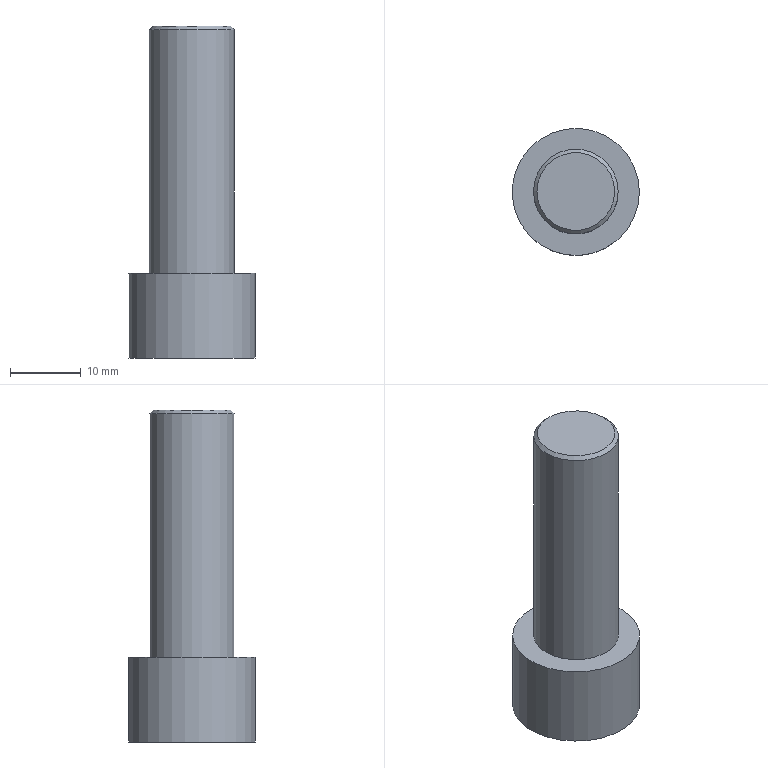Part | STEP file | 1_id58_xmt_txt | 1 solid | 19 faces | box 18 x 18 x 47 mm | volume 6453 mm3 | plane 15 | cylinder 2 | cone 2 | commonest cylinder face diameters 12 x1 18 x1
STEP:
#1=CARTESIAN_POINT('',(86.,-23.,-79.));
#2=VERTEX_POINT('',#1);
#3=CARTESIAN_POINT('',(77.,-23.,-79.));
#4=DIRECTION('',(0.,0.,-1.));
#5=DIRECTION('',(1.,0.,0.));
#6=AXIS2_PLACEMENT_3D('',#3,#4,#5);
#7=CIRCLE('',#6,9.);
#8=EDGE_CURVE('',#2,#2,#7,.T.);
#9=ORIENTED_EDGE('',*,*,#8,.F.);
#10=EDGE_LOOP('',(#9));
#11=FACE_BOUND('',#10,.T.);
#12=CARTESIAN_POINT('',(86.,-23.,-67.));
#13=VERTEX_POINT('',#12);
#14=CARTESIAN_POINT('',(77.,-23.,-67.));
#15=DIRECTION('',(0.,0.,1.));
#16=DIRECTION('',(1.,0.,0.));
#17=AXIS2_PLACEMENT_3D('',#14,#15,#16);
#18=CIRCLE('',#17,9.);
#19=EDGE_CURVE('',#13,#13,#18,.T.);
#20=ORIENTED_EDGE('',*,*,#19,.F.);
#21=EDGE_LOOP('',(#20));
#22=FACE_BOUND('',#21,.T.);
#23=CARTESIAN_POINT('',(77.,-23.,-73.));
#24=DIRECTION('',(0.,0.,1.));
#25=DIRECTION('',(-1.,0.,0.));
#26=AXIS2_PLACEMENT_3D('',#23,#24,#25);
#27=CYLINDRICAL_SURFACE('',#26,9.);
#28=ADVANCED_FACE('',(#11,#22),#27,.T.);
#29=CARTESIAN_POINT('',(77.,-17.226,-73.));
#30=VERTEX_POINT('',#29);
#31=CARTESIAN_POINT('',(82.,-20.113,-73.));
#32=VERTEX_POINT('',#31);
#33=CARTESIAN_POINT('',(77.,-23.,-73.));
#34=DIRECTION('',(0.,0.,-1.));
#35=DIRECTION('',(1.,0.,0.));
#36=AXIS2_PLACEMENT_3D('',#33,#34,#35);
#37=CIRCLE('',#36,5.774);
#38=EDGE_CURVE('',#30,#32,#37,.T.);
#39=ORIENTED_EDGE('',*,*,#38,.T.);
#40=CARTESIAN_POINT('',(82.,-25.887,-73.));
#41=VERTEX_POINT('',#40);
#42=CARTESIAN_POINT('',(77.,-23.,-73.));
#43=DIRECTION('',(0.,0.,-1.));
#44=DIRECTION('',(1.,0.,0.));
#45=AXIS2_PLACEMENT_3D('',#42,#43,#44);
#46=CIRCLE('',#45,5.774);
#47=EDGE_CURVE('',#32,#41,#46,.T.);
#48=ORIENTED_EDGE('',*,*,#47,.T.);
#49=CARTESIAN_POINT('',(77.,-28.774,-73.));
#50=VERTEX_POINT('',#49);
#51=CARTESIAN_POINT('',(77.,-23.,-73.));
#52=DIRECTION('',(0.,0.,-1.));
#53=DIRECTION('',(1.,0.,0.));
#54=AXIS2_PLACEMENT_3D('',#51,#52,#53);
#55=CIRCLE('',#54,5.774);
#56=EDGE_CURVE('',#41,#50,#55,.T.);
#57=ORIENTED_EDGE('',*,*,#56,.T.);
#58=CARTESIAN_POINT('',(72.,-25.887,-73.));
#59=VERTEX_POINT('',#58);
#60=CARTESIAN_POINT('',(77.,-23.,-73.));
#61=DIRECTION('',(0.,0.,-1.));
#62=DIRECTION('',(1.,0.,0.));
#63=AXIS2_PLACEMENT_3D('',#60,#61,#62);
#64=CIRCLE('',#63,5.774);
#65=EDGE_CURVE('',#50,#59,#64,.T.);
#66=ORIENTED_EDGE('',*,*,#65,.T.);
#67=CARTESIAN_POINT('',(72.,-20.113,-73.));
#68=VERTEX_POINT('',#67);
#69=CARTESIAN_POINT('',(77.,-23.,-73.));
#70=DIRECTION('',(0.,0.,-1.));
#71=DIRECTION('',(1.,0.,0.));
#72=AXIS2_PLACEMENT_3D('',#69,#70,#71);
#73=CIRCLE('',#72,5.774);
#74=EDGE_CURVE('',#59,#68,#73,.T.);
#75=ORIENTED_EDGE('',*,*,#74,.T.);
#76=CARTESIAN_POINT('',(77.,-23.,-73.));
#77=DIRECTION('',(0.,0.,-1.));
#78=DIRECTION('',(1.,0.,0.));
#79=AXIS2_PLACEMENT_3D('',#76,#77,#78);
#80=CIRCLE('',#79,5.774);
#81=EDGE_CURVE('',#68,#30,#80,.T.);
#82=ORIENTED_EDGE('',*,*,#81,.T.);
#83=EDGE_LOOP('',(#39,#48,#57,#66,#75,#82));
#84=FACE_BOUND('',#83,.T.);
#85=CARTESIAN_POINT('',(77.,-23.,-72.));
#86=VERTEX_POINT('',#85);
#87=VERTEX_LOOP('',#86);
#88=FACE_BOUND('',#87,.T.);
#89=CARTESIAN_POINT('',(77.,-23.,-72.5));
#90=DIRECTION('',(0.,0.,-1.));
#91=DIRECTION('',(-1.,0.,0.));
#92=AXIS2_PLACEMENT_3D('',#89,#90,#91);
#93=CONICAL_SURFACE('',#92,2.887,80.174);
#94=ADVANCED_FACE('',(#84,#88),#93,.F.);
#95=CARTESIAN_POINT('',(83.,-23.,-67.));
#96=VERTEX_POINT('',#95);
#97=CARTESIAN_POINT('',(77.,-23.,-67.));
#98=DIRECTION('',(0.,0.,-1.));
#99=DIRECTION('',(1.,0.,0.));
#100=AXIS2_PLACEMENT_3D('',#97,#98,#99);
#101=CIRCLE('',#100,6.);
#102=EDGE_CURVE('',#96,#96,#101,.T.);
#103=ORIENTED_EDGE('',*,*,#102,.F.);
#104=EDGE_LOOP('',(#103));
#105=FACE_BOUND('',#104,.T.);
#106=CARTESIAN_POINT('',(71.,-23.,-32.5));
#107=VERTEX_POINT('',#106);
#108=CARTESIAN_POINT('',(77.,-23.,-32.5));
#109=DIRECTION('',(0.,0.,1.));
#110=DIRECTION('',(-1.,0.,0.));
#111=AXIS2_PLACEMENT_3D('',#108,#109,#110);
#112=CIRCLE('',#111,6.);
#113=EDGE_CURVE('',#107,#107,#112,.T.);
#114=ORIENTED_EDGE('',*,*,#113,.F.);
#115=EDGE_LOOP('',(#114));
#116=FACE_BOUND('',#115,.T.);
#117=CARTESIAN_POINT('',(77.,-23.,-49.5));
#118=DIRECTION('',(0.,0.,1.));
#119=DIRECTION('',(-1.,0.,0.));
#120=AXIS2_PLACEMENT_3D('',#117,#118,#119);
#121=CYLINDRICAL_SURFACE('',#120,6.);
#122=ADVANCED_FACE('',(#105,#116),#121,.T.);
#123=ORIENTED_EDGE('',*,*,#113,.T.);
#124=EDGE_LOOP('',(#123));
#125=FACE_BOUND('',#124,.T.);
#126=CARTESIAN_POINT('',(71.5,-23.,-32.));
#127=VERTEX_POINT('',#126);
#128=CARTESIAN_POINT('',(77.,-23.,-32.));
#129=DIRECTION('',(0.,0.,-1.));
#130=DIRECTION('',(-1.,0.,0.));
#131=AXIS2_PLACEMENT_3D('',#128,#129,#130);
#132=CIRCLE('',#131,5.5);
#133=EDGE_CURVE('',#127,#127,#132,.T.);
#134=ORIENTED_EDGE('',*,*,#133,.T.);
#135=EDGE_LOOP('',(#134));
#136=FACE_BOUND('',#135,.T.);
#137=CARTESIAN_POINT('',(77.,-23.,-32.));
#138=DIRECTION('',(0.,0.,-1.));
#139=DIRECTION('',(1.,0.,0.));
#140=AXIS2_PLACEMENT_3D('',#137,#138,#139);
#141=CONICAL_SURFACE('',#140,5.5,45.);
#142=ADVANCED_FACE('',(#125,#136),#141,.T.);
#143=ORIENTED_EDGE('',*,*,#133,.F.);
#144=EDGE_LOOP('',(#143));
#145=FACE_OUTER_BOUND('',#144,.T.);
#146=CARTESIAN_POINT('',(77.,-23.,-32.));
#147=DIRECTION('',(0.,0.,1.));
#148=DIRECTION('',(-1.,0.,0.));
#149=AXIS2_PLACEMENT_3D('',#146,#147,#148);
#150=PLANE('',#149);
#151=ADVANCED_FACE('',(#145),#150,.T.);
#152=CARTESIAN_POINT('',(79.5,-27.33,-73.));
#153=DIRECTION('',(0.866,0.5,0.));
#154=VECTOR('',#153,1.);
#155=LINE('',#152,#154);
#156=EDGE_CURVE('',#50,#41,#155,.T.);
#157=ORIENTED_EDGE('',*,*,#156,.F.);
#158=ORIENTED_EDGE('',*,*,#56,.F.);
#159=EDGE_LOOP('',(#157,#158));
#160=FACE_OUTER_BOUND('',#159,.T.);
#161=CARTESIAN_POINT('',(77.,-23.,-73.));
#162=DIRECTION('',(0.,0.,-1.));
#163=DIRECTION('',(1.,0.,0.));
#164=AXIS2_PLACEMENT_3D('',#161,#162,#163);
#165=PLANE('',#164);
#166=ADVANCED_FACE('',(#160),#165,.F.);
#167=CARTESIAN_POINT('',(82.,-23.,-73.));
#168=DIRECTION('',(0.,1.,0.));
#169=VECTOR('',#168,1.);
#170=LINE('',#167,#169);
#171=EDGE_CURVE('',#41,#32,#170,.T.);
#172=ORIENTED_EDGE('',*,*,#171,.F.);
#173=ORIENTED_EDGE('',*,*,#47,.F.);
#174=EDGE_LOOP('',(#172,#173));
#175=FACE_OUTER_BOUND('',#174,.T.);
#176=CARTESIAN_POINT('',(77.,-23.,-73.));
#177=DIRECTION('',(0.,0.,-1.));
#178=DIRECTION('',(1.,0.,0.));
#179=AXIS2_PLACEMENT_3D('',#176,#177,#178);
#180=PLANE('',#179);
#181=ADVANCED_FACE('',(#175),#180,.F.);
#182=CARTESIAN_POINT('',(79.5,-18.67,-73.));
#183=DIRECTION('',(-0.866,0.5,0.));
#184=VECTOR('',#183,1.);
#185=LINE('',#182,#184);
#186=EDGE_CURVE('',#32,#30,#185,.T.);
#187=ORIENTED_EDGE('',*,*,#186,.F.);
#188=ORIENTED_EDGE('',*,*,#38,.F.);
#189=EDGE_LOOP('',(#187,#188));
#190=FACE_OUTER_BOUND('',#189,.T.);
#191=CARTESIAN_POINT('',(77.,-23.,-73.));
#192=DIRECTION('',(0.,0.,-1.));
#193=DIRECTION('',(1.,0.,0.));
#194=AXIS2_PLACEMENT_3D('',#191,#192,#193);
#195=PLANE('',#194);
#196=ADVANCED_FACE('',(#190),#195,.F.);
#197=CARTESIAN_POINT('',(74.5,-18.67,-73.));
#198=DIRECTION('',(-0.866,-0.5,0.));
#199=VECTOR('',#198,1.);
#200=LINE('',#197,#199);
#201=EDGE_CURVE('',#30,#68,#200,.T.);
#202=ORIENTED_EDGE('',*,*,#201,.F.);
#203=ORIENTED_EDGE('',*,*,#81,.F.);
#204=EDGE_LOOP('',(#202,#203));
#205=FACE_OUTER_BOUND('',#204,.T.);
#206=CARTESIAN_POINT('',(77.,-23.,-73.));
#207=DIRECTION('',(0.,0.,-1.));
#208=DIRECTION('',(1.,0.,0.));
#209=AXIS2_PLACEMENT_3D('',#206,#207,#208);
#210=PLANE('',#209);
#211=ADVANCED_FACE('',(#205),#210,.F.);
#212=CARTESIAN_POINT('',(72.,-23.,-73.));
#213=DIRECTION('',(0.,-1.,0.));
#214=VECTOR('',#213,1.);
#215=LINE('',#212,#214);
#216=EDGE_CURVE('',#68,#59,#215,.T.);
#217=ORIENTED_EDGE('',*,*,#216,.F.);
#218=ORIENTED_EDGE('',*,*,#74,.F.);
#219=EDGE_LOOP('',(#217,#218));
#220=FACE_OUTER_BOUND('',#219,.T.);
#221=CARTESIAN_POINT('',(77.,-23.,-73.));
#222=DIRECTION('',(0.,0.,-1.));
#223=DIRECTION('',(1.,0.,0.));
#224=AXIS2_PLACEMENT_3D('',#221,#222,#223);
#225=PLANE('',#224);
#226=ADVANCED_FACE('',(#220),#225,.F.);
#227=CARTESIAN_POINT('',(74.5,-27.33,-73.));
#228=DIRECTION('',(0.866,-0.5,0.));
#229=VECTOR('',#228,1.);
#230=LINE('',#227,#229);
#231=EDGE_CURVE('',#59,#50,#230,.T.);
#232=ORIENTED_EDGE('',*,*,#231,.F.);
#233=ORIENTED_EDGE('',*,*,#65,.F.);
#234=EDGE_LOOP('',(#232,#233));
#235=FACE_OUTER_BOUND('',#234,.T.);
#236=CARTESIAN_POINT('',(77.,-23.,-73.));
#237=DIRECTION('',(0.,0.,-1.));
#238=DIRECTION('',(1.,0.,0.));
#239=AXIS2_PLACEMENT_3D('',#236,#237,#238);
#240=PLANE('',#239);
#241=ADVANCED_FACE('',(#235),#240,.F.);
#242=CARTESIAN_POINT('',(77.,-28.774,-79.));
#243=VERTEX_POINT('',#242);
#244=CARTESIAN_POINT('',(77.,-28.774,-76.));
#245=DIRECTION('',(0.,0.,-1.));
#246=VECTOR('',#245,1.);
#247=LINE('',#244,#246);
#248=EDGE_CURVE('',#50,#243,#247,.T.);
#249=ORIENTED_EDGE('',*,*,#248,.F.);
#250=ORIENTED_EDGE('',*,*,#156,.T.);
#251=CARTESIAN_POINT('',(82.,-25.887,-79.));
#252=VERTEX_POINT('',#251);
#253=CARTESIAN_POINT('',(82.,-25.887,-76.));
#254=DIRECTION('',(0.,0.,-1.));
#255=VECTOR('',#254,1.);
#256=LINE('',#253,#255);
#257=EDGE_CURVE('',#41,#252,#256,.T.);
#258=ORIENTED_EDGE('',*,*,#257,.T.);
#259=CARTESIAN_POINT('',(79.5,-27.33,-79.));
#260=DIRECTION('',(0.866,0.5,0.));
#261=VECTOR('',#260,1.);
#262=LINE('',#259,#261);
#263=EDGE_CURVE('',#243,#252,#262,.T.);
#264=ORIENTED_EDGE('',*,*,#263,.F.);
#265=EDGE_LOOP('',(#249,#250,#258,#264));
#266=FACE_OUTER_BOUND('',#265,.T.);
#267=CARTESIAN_POINT('',(79.5,-27.33,-76.));
#268=DIRECTION('',(-0.5,0.866,0.));
#269=DIRECTION('',(0.,0.,-1.));
#270=AXIS2_PLACEMENT_3D('',#267,#268,#269);
#271=PLANE('',#270);
#272=ADVANCED_FACE('',(#266),#271,.T.);
#273=CARTESIAN_POINT('',(72.,-25.887,-79.));
#274=VERTEX_POINT('',#273);
#275=CARTESIAN_POINT('',(72.,-25.887,-76.));
#276=DIRECTION('',(0.,0.,-1.));
#277=VECTOR('',#276,1.);
#278=LINE('',#275,#277);
#279=EDGE_CURVE('',#59,#274,#278,.T.);
#280=ORIENTED_EDGE('',*,*,#279,.F.);
#281=ORIENTED_EDGE('',*,*,#231,.T.);
#282=ORIENTED_EDGE('',*,*,#248,.T.);
#283=CARTESIAN_POINT('',(74.5,-27.33,-79.));
#284=DIRECTION('',(0.866,-0.5,0.));
#285=VECTOR('',#284,1.);
#286=LINE('',#283,#285);
#287=EDGE_CURVE('',#274,#243,#286,.T.);
#288=ORIENTED_EDGE('',*,*,#287,.F.);
#289=EDGE_LOOP('',(#280,#281,#282,#288));
#290=FACE_OUTER_BOUND('',#289,.T.);
#291=CARTESIAN_POINT('',(74.5,-27.33,-76.));
#292=DIRECTION('',(0.5,0.866,0.));
#293=DIRECTION('',(0.,0.,1.));
#294=AXIS2_PLACEMENT_3D('',#291,#292,#293);
#295=PLANE('',#294);
#296=ADVANCED_FACE('',(#290),#295,.T.);
#297=CARTESIAN_POINT('',(72.,-20.113,-79.));
#298=VERTEX_POINT('',#297);
#299=CARTESIAN_POINT('',(72.,-20.113,-76.));
#300=DIRECTION('',(0.,0.,-1.));
#301=VECTOR('',#300,1.);
#302=LINE('',#299,#301);
#303=EDGE_CURVE('',#68,#298,#302,.T.);
#304=ORIENTED_EDGE('',*,*,#303,.F.);
#305=ORIENTED_EDGE('',*,*,#216,.T.);
#306=ORIENTED_EDGE('',*,*,#279,.T.);
#307=CARTESIAN_POINT('',(72.,-23.,-79.));
#308=DIRECTION('',(0.,-1.,0.));
#309=VECTOR('',#308,1.);
#310=LINE('',#307,#309);
#311=EDGE_CURVE('',#298,#274,#310,.T.);
#312=ORIENTED_EDGE('',*,*,#311,.F.);
#313=EDGE_LOOP('',(#304,#305,#306,#312));
#314=FACE_OUTER_BOUND('',#313,.T.);
#315=CARTESIAN_POINT('',(72.,-23.,-76.));
#316=DIRECTION('',(1.,0.,0.));
#317=DIRECTION('',(0.,0.,1.));
#318=AXIS2_PLACEMENT_3D('',#315,#316,#317);
#319=PLANE('',#318);
#320=ADVANCED_FACE('',(#314),#319,.T.);
#321=CARTESIAN_POINT('',(77.,-17.226,-79.));
#322=VERTEX_POINT('',#321);
#323=CARTESIAN_POINT('',(77.,-17.226,-76.));
#324=DIRECTION('',(0.,0.,-1.));
#325=VECTOR('',#324,1.);
#326=LINE('',#323,#325);
#327=EDGE_CURVE('',#30,#322,#326,.T.);
#328=ORIENTED_EDGE('',*,*,#327,.F.);
#329=ORIENTED_EDGE('',*,*,#201,.T.);
#330=ORIENTED_EDGE('',*,*,#303,.T.);
#331=CARTESIAN_POINT('',(74.5,-18.67,-79.));
#332=DIRECTION('',(-0.866,-0.5,0.));
#333=VECTOR('',#332,1.);
#334=LINE('',#331,#333);
#335=EDGE_CURVE('',#322,#298,#334,.T.);
#336=ORIENTED_EDGE('',*,*,#335,.F.);
#337=EDGE_LOOP('',(#328,#329,#330,#336));
#338=FACE_OUTER_BOUND('',#337,.T.);
#339=CARTESIAN_POINT('',(74.5,-18.67,-76.));
#340=DIRECTION('',(0.5,-0.866,0.));
#341=DIRECTION('',(0.,0.,1.));
#342=AXIS2_PLACEMENT_3D('',#339,#340,#341);
#343=PLANE('',#342);
#344=ADVANCED_FACE('',(#338),#343,.T.);
#345=CARTESIAN_POINT('',(82.,-20.113,-79.));
#346=VERTEX_POINT('',#345);
#347=CARTESIAN_POINT('',(82.,-20.113,-76.));
#348=DIRECTION('',(0.,0.,-1.));
#349=VECTOR('',#348,1.);
#350=LINE('',#347,#349);
#351=EDGE_CURVE('',#32,#346,#350,.T.);
#352=ORIENTED_EDGE('',*,*,#351,.F.);
#353=ORIENTED_EDGE('',*,*,#186,.T.);
#354=ORIENTED_EDGE('',*,*,#327,.T.);
#355=CARTESIAN_POINT('',(79.5,-18.67,-79.));
#356=DIRECTION('',(-0.866,0.5,0.));
#357=VECTOR('',#356,1.);
#358=LINE('',#355,#357);
#359=EDGE_CURVE('',#346,#322,#358,.T.);
#360=ORIENTED_EDGE('',*,*,#359,.F.);
#361=EDGE_LOOP('',(#352,#353,#354,#360));
#362=FACE_OUTER_BOUND('',#361,.T.);
#363=CARTESIAN_POINT('',(79.5,-18.67,-76.));
#364=DIRECTION('',(-0.5,-0.866,0.));
#365=DIRECTION('',(0.,0.,-1.));
#366=AXIS2_PLACEMENT_3D('',#363,#364,#365);
#367=PLANE('',#366);
#368=ADVANCED_FACE('',(#362),#367,.T.);
#369=ORIENTED_EDGE('',*,*,#257,.F.);
#370=ORIENTED_EDGE('',*,*,#171,.T.);
#371=ORIENTED_EDGE('',*,*,#351,.T.);
#372=CARTESIAN_POINT('',(82.,-23.,-79.));
#373=DIRECTION('',(0.,1.,0.));
#374=VECTOR('',#373,1.);
#375=LINE('',#372,#374);
#376=EDGE_CURVE('',#252,#346,#375,.T.);
#377=ORIENTED_EDGE('',*,*,#376,.F.);
#378=EDGE_LOOP('',(#369,#370,#371,#377));
#379=FACE_OUTER_BOUND('',#378,.T.);
#380=CARTESIAN_POINT('',(82.,-23.,-76.));
#381=DIRECTION('',(-1.,0.,0.));
#382=DIRECTION('',(0.,0.,-1.));
#383=AXIS2_PLACEMENT_3D('',#380,#381,#382);
#384=PLANE('',#383);
#385=ADVANCED_FACE('',(#379),#384,.T.);
#386=ORIENTED_EDGE('',*,*,#263,.T.);
#387=ORIENTED_EDGE('',*,*,#376,.T.);
#388=ORIENTED_EDGE('',*,*,#359,.T.);
#389=ORIENTED_EDGE('',*,*,#335,.T.);
#390=ORIENTED_EDGE('',*,*,#311,.T.);
#391=ORIENTED_EDGE('',*,*,#287,.T.);
#392=EDGE_LOOP('',(#386,#387,#388,#389,#390,#391));
#393=FACE_BOUND('',#392,.T.);
#394=ORIENTED_EDGE('',*,*,#8,.T.);
#395=EDGE_LOOP('',(#394));
#396=FACE_BOUND('',#395,.T.);
#397=CARTESIAN_POINT('',(77.,-23.,-79.));
#398=DIRECTION('',(0.,0.,-1.));
#399=DIRECTION('',(1.,0.,0.));
#400=AXIS2_PLACEMENT_3D('',#397,#398,#399);
#401=PLANE('',#400);
#402=ADVANCED_FACE('',(#393,#396),#401,.T.);
#403=ORIENTED_EDGE('',*,*,#102,.T.);
#404=EDGE_LOOP('',(#403));
#405=FACE_BOUND('',#404,.T.);
#406=ORIENTED_EDGE('',*,*,#19,.T.);
#407=EDGE_LOOP('',(#406));
#408=FACE_BOUND('',#407,.T.);
#409=CARTESIAN_POINT('',(77.,-23.,-67.));
#410=DIRECTION('',(0.,0.,1.));
#411=DIRECTION('',(-1.,0.,0.));
#412=AXIS2_PLACEMENT_3D('',#409,#410,#411);
#413=PLANE('',#412);
#414=ADVANCED_FACE('',(#405,#408),#413,.T.);
#415=CLOSED_SHELL('',(#28,#94,#122,#142,#151,#166,#181,#196,#211,#226,#241,#272,#296,#320,#344,#368,#385,#402,#414));
#416=MANIFOLD_SOLID_BREP('',#415);
#417=(LENGTH_UNIT()NAMED_UNIT(*)SI_UNIT(.MILLI.,.METRE.));
#418=UNCERTAINTY_MEASURE_WITH_UNIT(LENGTH_MEASURE(0.00002),#417,'','');
#419=(NAMED_UNIT(*)PLANE_ANGLE_UNIT()SI_UNIT($,.RADIAN.));
#420=PLANE_ANGLE_MEASURE_WITH_UNIT(PLANE_ANGLE_MEASURE(0.01745),#419);
#421=DIMENSIONAL_EXPONENTS(0.,0.,0.,0.,0.,0.,0.);
#422=(CONVERSION_BASED_UNIT('DEGREE',#420)NAMED_UNIT(#421)PLANE_ANGLE_UNIT());
#423=(NAMED_UNIT(*)SI_UNIT($,.STERADIAN.)SOLID_ANGLE_UNIT());
#424=(GEOMETRIC_REPRESENTATION_CONTEXT(3)GLOBAL_UNCERTAINTY_ASSIGNED_CONTEXT((#418))GLOBAL_UNIT_ASSIGNED_CONTEXT((#417,#422,#423))REPRESENTATION_CONTEXT('',''));
#425=ADVANCED_BREP_SHAPE_REPRESENTATION('',(#416),#424);